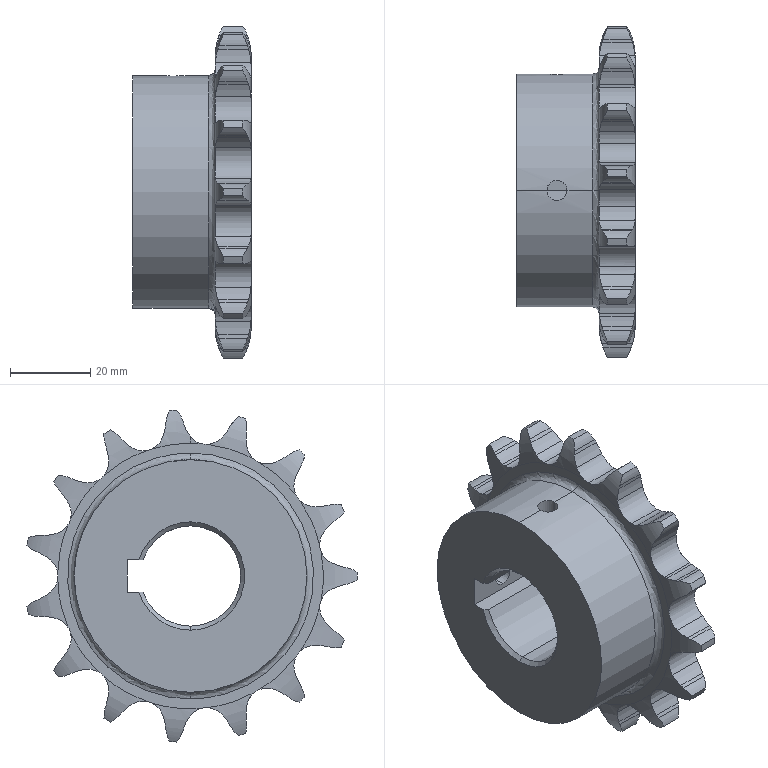Part | STEP file | 1 solid | 179 faces | box 29.497 x 82.28 x 82.723 mm | volume 74785 mm3 | cylinder 105 | plane 36 | spline 34 | cone 4 | commonest cylinder face diameters 14.954 x31 26.567 x31 10.311 x19 83 x15 5 x4 25 x3